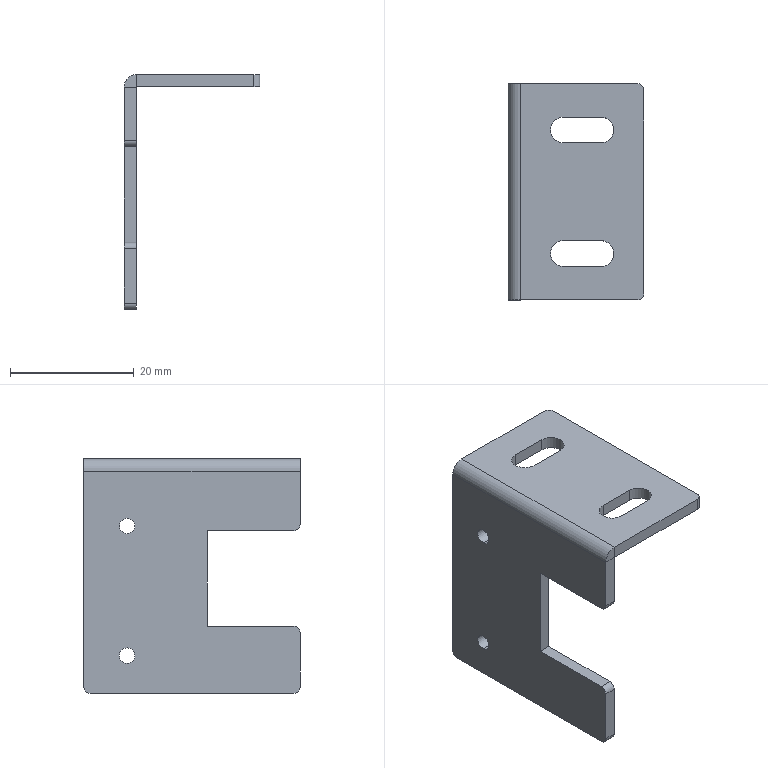Part | STEP file | photoelectric mounting plate | 1 solid | 38 faces | box 22 x 35 x 38 mm | volume 3386 mm3 | plane 20 | cylinder 18 | commonest cylinder face diameters 2 x6 4.2 x6 2.5 x4 0.02 x1 4.02 x1